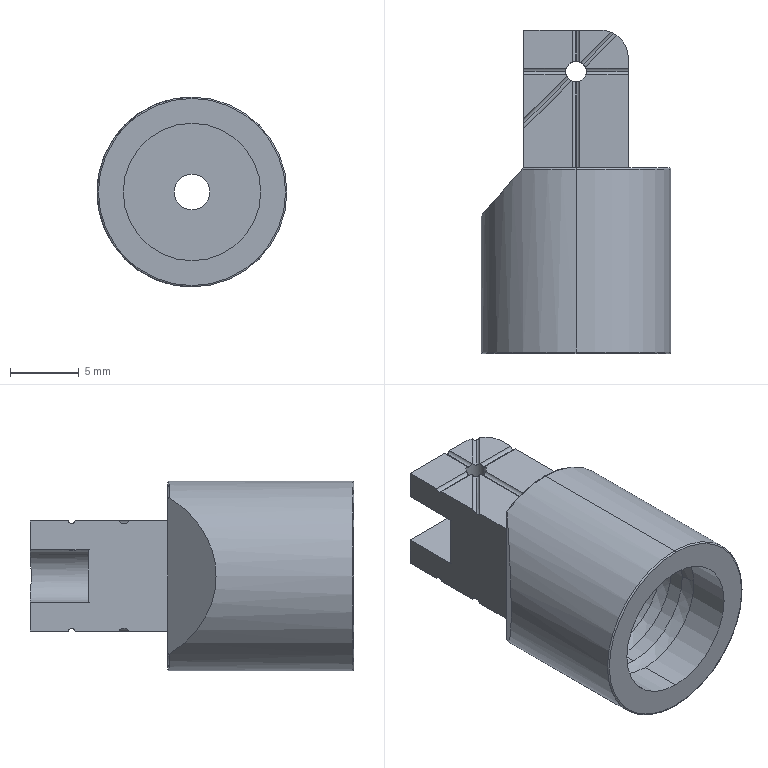Part | SolidWorks | features ICE 7, Fillet 2, MirrorPattern 1, Revolution 1 | 1 solid | 87 faces | box 13.8 x 23.5 x 13.8 mm | volume 1561 mm3 | cylinder 40 | plane 38 | torus 5 | spline 4 | commonest cylinder face diameters 0.51 x24 10 x6 1.5 x4 2.6 x2 13.8 x2 3.85 x1